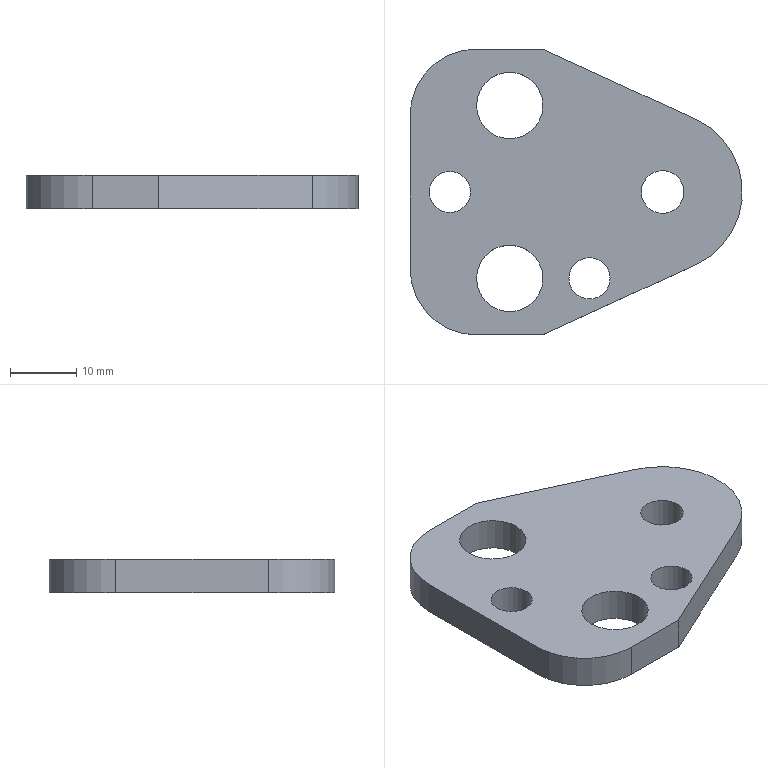Part | NX | features solid 2 | 1 solid | 15 faces | box 50 x 43 x 5 mm | volume 7113 mm3 | cylinder 8 | plane 7 | commonest cylinder face diameters 6.2 x2 10 x2 20 x2 6.4 x1 24 x1
STEP:
#1=CARTESIAN_POINT('',(-1290.413,363.428,133.));
#2=VERTEX_POINT('',#1);
#3=CARTESIAN_POINT('',(-1300.413,373.428,133.));
#4=VERTEX_POINT('',#3);
#5=CARTESIAN_POINT('',(-1290.413,373.428,133.));
#6=DIRECTION('',(0.,0.,-1.));
#7=DIRECTION('',(-1.,0.,0.));
#8=AXIS2_PLACEMENT_3D('',#5,#6,#7);
#9=CIRCLE('',#8,10.);
#10=EDGE_CURVE('',#2,#4,#9,.T.);
#11=ORIENTED_EDGE('',*,*,#10,.F.);
#12=CARTESIAN_POINT('',(-1290.413,363.428,138.));
#13=VERTEX_POINT('',#12);
#14=CARTESIAN_POINT('',(-1290.413,363.428,138.));
#15=DIRECTION('',(0.,0.,-1.));
#16=VECTOR('',#15,1000.);
#17=LINE('',#14,#16);
#18=EDGE_CURVE('',#13,#2,#17,.T.);
#19=ORIENTED_EDGE('',*,*,#18,.F.);
#20=CARTESIAN_POINT('',(-1300.413,373.428,138.));
#21=VERTEX_POINT('',#20);
#22=CARTESIAN_POINT('',(-1290.413,373.428,138.));
#23=DIRECTION('',(0.,0.,-1.));
#24=DIRECTION('',(-1.,0.,0.));
#25=AXIS2_PLACEMENT_3D('',#22,#23,#24);
#26=CIRCLE('',#25,10.);
#27=EDGE_CURVE('',#13,#21,#26,.T.);
#28=ORIENTED_EDGE('',*,*,#27,.T.);
#29=CARTESIAN_POINT('',(-1300.413,373.428,138.));
#30=DIRECTION('',(0.,0.,-1.));
#31=VECTOR('',#30,1000.);
#32=LINE('',#29,#31);
#33=EDGE_CURVE('',#21,#4,#32,.T.);
#34=ORIENTED_EDGE('',*,*,#33,.T.);
#35=EDGE_LOOP('',(#11,#19,#28,#34));
#36=FACE_BOUND('',#35,.T.);
#37=CARTESIAN_POINT('',(-1290.413,373.428,138.));
#38=DIRECTION('',(0.,0.,-1.));
#39=DIRECTION('',(-1.,0.,0.));
#40=AXIS2_PLACEMENT_3D('',#37,#38,#39);
#41=CYLINDRICAL_SURFACE('',#40,10.);
#42=ADVANCED_FACE('',(#36),#41,.T.);
#43=CARTESIAN_POINT('',(-1300.413,396.428,133.));
#44=VERTEX_POINT('',#43);
#45=CARTESIAN_POINT('',(-1300.413,396.428,133.));
#46=DIRECTION('',(0.,-1.,0.));
#47=VECTOR('',#46,1000.);
#48=LINE('',#45,#47);
#49=EDGE_CURVE('',#44,#4,#48,.T.);
#50=ORIENTED_EDGE('',*,*,#49,.T.);
#51=ORIENTED_EDGE('',*,*,#33,.F.);
#52=CARTESIAN_POINT('',(-1300.413,396.428,138.));
#53=VERTEX_POINT('',#52);
#54=CARTESIAN_POINT('',(-1300.413,396.428,138.));
#55=DIRECTION('',(0.,-1.,0.));
#56=VECTOR('',#55,1000.);
#57=LINE('',#54,#56);
#58=EDGE_CURVE('',#53,#21,#57,.T.);
#59=ORIENTED_EDGE('',*,*,#58,.F.);
#60=CARTESIAN_POINT('',(-1300.413,396.428,138.));
#61=DIRECTION('',(0.,0.,-1.));
#62=VECTOR('',#61,1000.);
#63=LINE('',#60,#62);
#64=EDGE_CURVE('',#53,#44,#63,.T.);
#65=ORIENTED_EDGE('',*,*,#64,.T.);
#66=EDGE_LOOP('',(#50,#51,#59,#65));
#67=FACE_BOUND('',#66,.T.);
#68=CARTESIAN_POINT('',(-1300.413,396.428,138.));
#69=DIRECTION('',(1.,0.,0.));
#70=DIRECTION('',(0.,1.,0.));
#71=AXIS2_PLACEMENT_3D('',#68,#69,#70);
#72=PLANE('',#71);
#73=ADVANCED_FACE('',(#67),#72,.F.);
#74=CARTESIAN_POINT('',(-1290.413,406.428,133.));
#75=VERTEX_POINT('',#74);
#76=CARTESIAN_POINT('',(-1290.413,396.428,133.));
#77=DIRECTION('',(0.,0.,-1.));
#78=DIRECTION('',(-1.,0.,0.));
#79=AXIS2_PLACEMENT_3D('',#76,#77,#78);
#80=CIRCLE('',#79,10.);
#81=EDGE_CURVE('',#44,#75,#80,.T.);
#82=ORIENTED_EDGE('',*,*,#81,.F.);
#83=ORIENTED_EDGE('',*,*,#64,.F.);
#84=CARTESIAN_POINT('',(-1290.413,406.428,138.));
#85=VERTEX_POINT('',#84);
#86=CARTESIAN_POINT('',(-1290.413,396.428,138.));
#87=DIRECTION('',(0.,0.,-1.));
#88=DIRECTION('',(-1.,0.,0.));
#89=AXIS2_PLACEMENT_3D('',#86,#87,#88);
#90=CIRCLE('',#89,10.);
#91=EDGE_CURVE('',#53,#85,#90,.T.);
#92=ORIENTED_EDGE('',*,*,#91,.T.);
#93=CARTESIAN_POINT('',(-1290.413,406.428,138.));
#94=DIRECTION('',(0.,0.,-1.));
#95=VECTOR('',#94,1000.);
#96=LINE('',#93,#95);
#97=EDGE_CURVE('',#85,#75,#96,.T.);
#98=ORIENTED_EDGE('',*,*,#97,.T.);
#99=EDGE_LOOP('',(#82,#83,#92,#98));
#100=FACE_BOUND('',#99,.T.);
#101=CARTESIAN_POINT('',(-1290.413,396.428,138.));
#102=DIRECTION('',(0.,0.,-1.));
#103=DIRECTION('',(-1.,0.,0.));
#104=AXIS2_PLACEMENT_3D('',#101,#102,#103);
#105=CYLINDRICAL_SURFACE('',#104,10.);
#106=ADVANCED_FACE('',(#100),#105,.T.);
#107=CARTESIAN_POINT('',(-1280.413,406.428,133.));
#108=VERTEX_POINT('',#107);
#109=CARTESIAN_POINT('',(-1280.413,406.428,133.));
#110=DIRECTION('',(-1.,0.,0.));
#111=VECTOR('',#110,1000.);
#112=LINE('',#109,#111);
#113=EDGE_CURVE('',#108,#75,#112,.T.);
#114=ORIENTED_EDGE('',*,*,#113,.T.);
#115=ORIENTED_EDGE('',*,*,#97,.F.);
#116=CARTESIAN_POINT('',(-1280.413,406.428,138.));
#117=VERTEX_POINT('',#116);
#118=CARTESIAN_POINT('',(-1280.413,406.428,138.));
#119=DIRECTION('',(-1.,0.,0.));
#120=VECTOR('',#119,1000.);
#121=LINE('',#118,#120);
#122=EDGE_CURVE('',#117,#85,#121,.T.);
#123=ORIENTED_EDGE('',*,*,#122,.F.);
#124=CARTESIAN_POINT('',(-1280.413,406.428,138.));
#125=DIRECTION('',(0.,0.,-1.));
#126=VECTOR('',#125,1000.);
#127=LINE('',#124,#126);
#128=EDGE_CURVE('',#117,#108,#127,.T.);
#129=ORIENTED_EDGE('',*,*,#128,.T.);
#130=EDGE_LOOP('',(#114,#115,#123,#129));
#131=FACE_BOUND('',#130,.T.);
#132=CARTESIAN_POINT('',(-1280.413,406.428,138.));
#133=DIRECTION('',(0.,-1.,0.));
#134=DIRECTION('',(1.,0.,0.));
#135=AXIS2_PLACEMENT_3D('',#132,#133,#134);
#136=PLANE('',#135);
#137=ADVANCED_FACE('',(#131),#136,.F.);
#138=CARTESIAN_POINT('',(-1257.394,395.828,133.));
#139=VERTEX_POINT('',#138);
#140=CARTESIAN_POINT('',(-1257.394,395.828,133.));
#141=DIRECTION('',(-0.9083,0.4183,0.));
#142=VECTOR('',#141,1000.);
#143=LINE('',#140,#142);
#144=EDGE_CURVE('',#139,#108,#143,.T.);
#145=ORIENTED_EDGE('',*,*,#144,.T.);
#146=ORIENTED_EDGE('',*,*,#128,.F.);
#147=CARTESIAN_POINT('',(-1257.394,395.828,138.));
#148=VERTEX_POINT('',#147);
#149=CARTESIAN_POINT('',(-1257.394,395.828,138.));
#150=DIRECTION('',(-0.9083,0.4183,0.));
#151=VECTOR('',#150,1000.);
#152=LINE('',#149,#151);
#153=EDGE_CURVE('',#148,#117,#152,.T.);
#154=ORIENTED_EDGE('',*,*,#153,.F.);
#155=CARTESIAN_POINT('',(-1257.394,395.828,138.));
#156=DIRECTION('',(0.,0.,-1.));
#157=VECTOR('',#156,1000.);
#158=LINE('',#155,#157);
#159=EDGE_CURVE('',#148,#139,#158,.T.);
#160=ORIENTED_EDGE('',*,*,#159,.T.);
#161=EDGE_LOOP('',(#145,#146,#154,#160));
#162=FACE_BOUND('',#161,.T.);
#163=CARTESIAN_POINT('',(-1257.394,395.828,138.));
#164=DIRECTION('',(-0.4183,-0.9083,0.));
#165=DIRECTION('',(0.9083,-0.4183,0.));
#166=AXIS2_PLACEMENT_3D('',#163,#164,#165);
#167=PLANE('',#166);
#168=ADVANCED_FACE('',(#162),#167,.F.);
#169=CARTESIAN_POINT('',(-1257.394,374.028,133.));
#170=VERTEX_POINT('',#169);
#171=CARTESIAN_POINT('',(-1262.413,384.928,133.));
#172=DIRECTION('',(0.,0.,-1.));
#173=DIRECTION('',(-1.,0.,0.));
#174=AXIS2_PLACEMENT_3D('',#171,#172,#173);
#175=CIRCLE('',#174,12.);
#176=EDGE_CURVE('',#139,#170,#175,.T.);
#177=ORIENTED_EDGE('',*,*,#176,.F.);
#178=ORIENTED_EDGE('',*,*,#159,.F.);
#179=CARTESIAN_POINT('',(-1257.394,374.028,138.));
#180=VERTEX_POINT('',#179);
#181=CARTESIAN_POINT('',(-1262.413,384.928,138.));
#182=DIRECTION('',(0.,0.,-1.));
#183=DIRECTION('',(-1.,0.,0.));
#184=AXIS2_PLACEMENT_3D('',#181,#182,#183);
#185=CIRCLE('',#184,12.);
#186=EDGE_CURVE('',#148,#180,#185,.T.);
#187=ORIENTED_EDGE('',*,*,#186,.T.);
#188=CARTESIAN_POINT('',(-1257.394,374.028,138.));
#189=DIRECTION('',(0.,0.,-1.));
#190=VECTOR('',#189,1000.);
#191=LINE('',#188,#190);
#192=EDGE_CURVE('',#180,#170,#191,.T.);
#193=ORIENTED_EDGE('',*,*,#192,.T.);
#194=EDGE_LOOP('',(#177,#178,#187,#193));
#195=FACE_BOUND('',#194,.T.);
#196=CARTESIAN_POINT('',(-1262.413,384.928,138.));
#197=DIRECTION('',(0.,0.,-1.));
#198=DIRECTION('',(-1.,0.,0.));
#199=AXIS2_PLACEMENT_3D('',#196,#197,#198);
#200=CYLINDRICAL_SURFACE('',#199,12.);
#201=ADVANCED_FACE('',(#195),#200,.T.);
#202=CARTESIAN_POINT('',(-1280.413,363.428,133.));
#203=VERTEX_POINT('',#202);
#204=CARTESIAN_POINT('',(-1257.394,374.028,133.));
#205=DIRECTION('',(-0.9083,-0.4183,0.));
#206=VECTOR('',#205,1000.);
#207=LINE('',#204,#206);
#208=EDGE_CURVE('',#170,#203,#207,.T.);
#209=ORIENTED_EDGE('',*,*,#208,.F.);
#210=ORIENTED_EDGE('',*,*,#192,.F.);
#211=CARTESIAN_POINT('',(-1280.413,363.428,138.));
#212=VERTEX_POINT('',#211);
#213=CARTESIAN_POINT('',(-1257.394,374.028,138.));
#214=DIRECTION('',(-0.9083,-0.4183,0.));
#215=VECTOR('',#214,1000.);
#216=LINE('',#213,#215);
#217=EDGE_CURVE('',#180,#212,#216,.T.);
#218=ORIENTED_EDGE('',*,*,#217,.T.);
#219=CARTESIAN_POINT('',(-1280.413,363.428,138.));
#220=DIRECTION('',(0.,0.,-1.));
#221=VECTOR('',#220,1000.);
#222=LINE('',#219,#221);
#223=EDGE_CURVE('',#212,#203,#222,.T.);
#224=ORIENTED_EDGE('',*,*,#223,.T.);
#225=EDGE_LOOP('',(#209,#210,#218,#224));
#226=FACE_BOUND('',#225,.T.);
#227=CARTESIAN_POINT('',(-1257.394,374.028,138.));
#228=DIRECTION('',(0.4183,-0.9083,0.));
#229=DIRECTION('',(0.9083,0.4183,0.));
#230=AXIS2_PLACEMENT_3D('',#227,#228,#229);
#231=PLANE('',#230);
#232=ADVANCED_FACE('',(#226),#231,.T.);
#233=CARTESIAN_POINT('',(-1280.413,363.428,133.));
#234=DIRECTION('',(-1.,0.,0.));
#235=VECTOR('',#234,1000.);
#236=LINE('',#233,#235);
#237=EDGE_CURVE('',#203,#2,#236,.T.);
#238=ORIENTED_EDGE('',*,*,#237,.F.);
#239=ORIENTED_EDGE('',*,*,#223,.F.);
#240=CARTESIAN_POINT('',(-1280.413,363.428,138.));
#241=DIRECTION('',(-1.,0.,0.));
#242=VECTOR('',#241,1000.);
#243=LINE('',#240,#242);
#244=EDGE_CURVE('',#212,#13,#243,.T.);
#245=ORIENTED_EDGE('',*,*,#244,.T.);
#246=ORIENTED_EDGE('',*,*,#18,.T.);
#247=EDGE_LOOP('',(#238,#239,#245,#246));
#248=FACE_BOUND('',#247,.T.);
#249=CARTESIAN_POINT('',(-1280.413,363.428,138.));
#250=DIRECTION('',(0.,-1.,0.));
#251=DIRECTION('',(1.,0.,0.));
#252=AXIS2_PLACEMENT_3D('',#249,#250,#251);
#253=PLANE('',#252);
#254=ADVANCED_FACE('',(#248),#253,.T.);
#255=CARTESIAN_POINT('',(-1290.413,397.928,138.));
#256=VERTEX_POINT('',#255);
#257=CARTESIAN_POINT('',(-1285.413,397.928,138.));
#258=DIRECTION('',(0.,0.,-1.));
#259=DIRECTION('',(-1.,0.,0.));
#260=AXIS2_PLACEMENT_3D('',#257,#258,#259);
#261=CIRCLE('',#260,5.);
#262=EDGE_CURVE('',#256,#256,#261,.T.);
#263=ORIENTED_EDGE('',*,*,#262,.T.);
#264=EDGE_LOOP('',(#263));
#265=FACE_BOUND('',#264,.T.);
#266=CARTESIAN_POINT('',(-1290.413,371.928,138.));
#267=VERTEX_POINT('',#266);
#268=CARTESIAN_POINT('',(-1285.413,371.928,138.));
#269=DIRECTION('',(0.,0.,-1.));
#270=DIRECTION('',(-1.,0.,0.));
#271=AXIS2_PLACEMENT_3D('',#268,#269,#270);
#272=CIRCLE('',#271,5.);
#273=EDGE_CURVE('',#267,#267,#272,.T.);
#274=ORIENTED_EDGE('',*,*,#273,.T.);
#275=EDGE_LOOP('',(#274));
#276=FACE_BOUND('',#275,.T.);
#277=CARTESIAN_POINT('',(-1265.613,384.928,138.));
#278=VERTEX_POINT('',#277);
#279=CARTESIAN_POINT('',(-1262.413,384.928,138.));
#280=DIRECTION('',(0.,0.,-1.));
#281=DIRECTION('',(-1.,0.,0.));
#282=AXIS2_PLACEMENT_3D('',#279,#280,#281);
#283=CIRCLE('',#282,3.2);
#284=EDGE_CURVE('',#278,#278,#283,.T.);
#285=ORIENTED_EDGE('',*,*,#284,.T.);
#286=EDGE_LOOP('',(#285));
#287=FACE_BOUND('',#286,.T.);
#288=CARTESIAN_POINT('',(-1276.513,371.928,138.));
#289=VERTEX_POINT('',#288);
#290=CARTESIAN_POINT('',(-1273.413,371.928,138.));
#291=DIRECTION('',(0.,0.,-1.));
#292=DIRECTION('',(-1.,0.,0.));
#293=AXIS2_PLACEMENT_3D('',#290,#291,#292);
#294=CIRCLE('',#293,3.1);
#295=EDGE_CURVE('',#289,#289,#294,.T.);
#296=ORIENTED_EDGE('',*,*,#295,.T.);
#297=EDGE_LOOP('',(#296));
#298=FACE_BOUND('',#297,.T.);
#299=CARTESIAN_POINT('',(-1297.513,384.928,138.));
#300=VERTEX_POINT('',#299);
#301=CARTESIAN_POINT('',(-1294.413,384.928,138.));
#302=DIRECTION('',(0.,0.,-1.));
#303=DIRECTION('',(-1.,0.,0.));
#304=AXIS2_PLACEMENT_3D('',#301,#302,#303);
#305=CIRCLE('',#304,3.1);
#306=EDGE_CURVE('',#300,#300,#305,.T.);
#307=ORIENTED_EDGE('',*,*,#306,.T.);
#308=EDGE_LOOP('',(#307));
#309=FACE_BOUND('',#308,.T.);
#310=ORIENTED_EDGE('',*,*,#27,.F.);
#311=ORIENTED_EDGE('',*,*,#244,.F.);
#312=ORIENTED_EDGE('',*,*,#217,.F.);
#313=ORIENTED_EDGE('',*,*,#186,.F.);
#314=ORIENTED_EDGE('',*,*,#153,.T.);
#315=ORIENTED_EDGE('',*,*,#122,.T.);
#316=ORIENTED_EDGE('',*,*,#91,.F.);
#317=ORIENTED_EDGE('',*,*,#58,.T.);
#318=EDGE_LOOP('',(#310,#311,#312,#313,#314,#315,#316,#317));
#319=FACE_BOUND('',#318,.T.);
#320=CARTESIAN_POINT('',(-1290.413,373.428,138.));
#321=DIRECTION('',(0.,0.,-1.));
#322=DIRECTION('',(-1.,0.,0.));
#323=AXIS2_PLACEMENT_3D('',#320,#321,#322);
#324=PLANE('',#323);
#325=ADVANCED_FACE('',(#265,#276,#287,#298,#309,#319),#324,.F.);
#326=CARTESIAN_POINT('',(-1290.413,397.928,133.));
#327=VERTEX_POINT('',#326);
#328=CARTESIAN_POINT('',(-1285.413,397.928,133.));
#329=DIRECTION('',(0.,0.,-1.));
#330=DIRECTION('',(-1.,0.,0.));
#331=AXIS2_PLACEMENT_3D('',#328,#329,#330);
#332=CIRCLE('',#331,5.);
#333=EDGE_CURVE('',#327,#327,#332,.T.);
#334=ORIENTED_EDGE('',*,*,#333,.F.);
#335=EDGE_LOOP('',(#334));
#336=FACE_BOUND('',#335,.T.);
#337=CARTESIAN_POINT('',(-1290.413,371.928,133.));
#338=VERTEX_POINT('',#337);
#339=CARTESIAN_POINT('',(-1285.413,371.928,133.));
#340=DIRECTION('',(0.,0.,-1.));
#341=DIRECTION('',(-1.,0.,0.));
#342=AXIS2_PLACEMENT_3D('',#339,#340,#341);
#343=CIRCLE('',#342,5.);
#344=EDGE_CURVE('',#338,#338,#343,.T.);
#345=ORIENTED_EDGE('',*,*,#344,.F.);
#346=EDGE_LOOP('',(#345));
#347=FACE_BOUND('',#346,.T.);
#348=CARTESIAN_POINT('',(-1265.613,384.928,133.));
#349=VERTEX_POINT('',#348);
#350=CARTESIAN_POINT('',(-1262.413,384.928,133.));
#351=DIRECTION('',(0.,0.,-1.));
#352=DIRECTION('',(-1.,0.,0.));
#353=AXIS2_PLACEMENT_3D('',#350,#351,#352);
#354=CIRCLE('',#353,3.2);
#355=EDGE_CURVE('',#349,#349,#354,.T.);
#356=ORIENTED_EDGE('',*,*,#355,.F.);
#357=EDGE_LOOP('',(#356));
#358=FACE_BOUND('',#357,.T.);
#359=CARTESIAN_POINT('',(-1276.513,371.928,133.));
#360=VERTEX_POINT('',#359);
#361=CARTESIAN_POINT('',(-1273.413,371.928,133.));
#362=DIRECTION('',(0.,0.,-1.));
#363=DIRECTION('',(-1.,0.,0.));
#364=AXIS2_PLACEMENT_3D('',#361,#362,#363);
#365=CIRCLE('',#364,3.1);
#366=EDGE_CURVE('',#360,#360,#365,.T.);
#367=ORIENTED_EDGE('',*,*,#366,.F.);
#368=EDGE_LOOP('',(#367));
#369=FACE_BOUND('',#368,.T.);
#370=CARTESIAN_POINT('',(-1297.513,384.928,133.));
#371=VERTEX_POINT('',#370);
#372=CARTESIAN_POINT('',(-1294.413,384.928,133.));
#373=DIRECTION('',(0.,0.,-1.));
#374=DIRECTION('',(-1.,0.,0.));
#375=AXIS2_PLACEMENT_3D('',#372,#373,#374);
#376=CIRCLE('',#375,3.1);
#377=EDGE_CURVE('',#371,#371,#376,.T.);
#378=ORIENTED_EDGE('',*,*,#377,.F.);
#379=EDGE_LOOP('',(#378));
#380=FACE_BOUND('',#379,.T.);
#381=ORIENTED_EDGE('',*,*,#10,.T.);
#382=ORIENTED_EDGE('',*,*,#49,.F.);
#383=ORIENTED_EDGE('',*,*,#81,.T.);
#384=ORIENTED_EDGE('',*,*,#113,.F.);
#385=ORIENTED_EDGE('',*,*,#144,.F.);
#386=ORIENTED_EDGE('',*,*,#176,.T.);
#387=ORIENTED_EDGE('',*,*,#208,.T.);
#388=ORIENTED_EDGE('',*,*,#237,.T.);
#389=EDGE_LOOP('',(#381,#382,#383,#384,#385,#386,#387,#388));
#390=FACE_BOUND('',#389,.T.);
#391=CARTESIAN_POINT('',(-1290.413,373.428,133.));
#392=DIRECTION('',(0.,0.,-1.));
#393=DIRECTION('',(-1.,0.,0.));
#394=AXIS2_PLACEMENT_3D('',#391,#392,#393);
#395=PLANE('',#394);
#396=ADVANCED_FACE('',(#336,#347,#358,#369,#380,#390),#395,.T.);
#397=ORIENTED_EDGE('',*,*,#377,.T.);
#398=EDGE_LOOP('',(#397));
#399=FACE_BOUND('',#398,.T.);
#400=ORIENTED_EDGE('',*,*,#306,.F.);
#401=EDGE_LOOP('',(#400));
#402=FACE_BOUND('',#401,.T.);
#403=CARTESIAN_POINT('',(-1294.413,384.928,138.));
#404=DIRECTION('',(0.,0.,-1.));
#405=DIRECTION('',(-1.,0.,0.));
#406=AXIS2_PLACEMENT_3D('',#403,#404,#405);
#407=CYLINDRICAL_SURFACE('',#406,3.1);
#408=ADVANCED_FACE('',(#399,#402),#407,.F.);
#409=ORIENTED_EDGE('',*,*,#366,.T.);
#410=EDGE_LOOP('',(#409));
#411=FACE_BOUND('',#410,.T.);
#412=ORIENTED_EDGE('',*,*,#295,.F.);
#413=EDGE_LOOP('',(#412));
#414=FACE_BOUND('',#413,.T.);
#415=CARTESIAN_POINT('',(-1273.413,371.928,138.));
#416=DIRECTION('',(0.,0.,-1.));
#417=DIRECTION('',(-1.,0.,0.));
#418=AXIS2_PLACEMENT_3D('',#415,#416,#417);
#419=CYLINDRICAL_SURFACE('',#418,3.1);
#420=ADVANCED_FACE('',(#411,#414),#419,.F.);
#421=ORIENTED_EDGE('',*,*,#355,.T.);
#422=EDGE_LOOP('',(#421));
#423=FACE_BOUND('',#422,.T.);
#424=ORIENTED_EDGE('',*,*,#284,.F.);
#425=EDGE_LOOP('',(#424));
#426=FACE_BOUND('',#425,.T.);
#427=CARTESIAN_POINT('',(-1262.413,384.928,138.));
#428=DIRECTION('',(0.,0.,-1.));
#429=DIRECTION('',(-1.,0.,0.));
#430=AXIS2_PLACEMENT_3D('',#427,#428,#429);
#431=CYLINDRICAL_SURFACE('',#430,3.2);
#432=ADVANCED_FACE('',(#423,#426),#431,.F.);
#433=ORIENTED_EDGE('',*,*,#344,.T.);
#434=EDGE_LOOP('',(#433));
#435=FACE_BOUND('',#434,.T.);
#436=ORIENTED_EDGE('',*,*,#273,.F.);
#437=EDGE_LOOP('',(#436));
#438=FACE_BOUND('',#437,.T.);
#439=CARTESIAN_POINT('',(-1285.413,371.928,138.));
#440=DIRECTION('',(0.,0.,-1.));
#441=DIRECTION('',(-1.,0.,0.));
#442=AXIS2_PLACEMENT_3D('',#439,#440,#441);
#443=CYLINDRICAL_SURFACE('',#442,5.);
#444=ADVANCED_FACE('',(#435,#438),#443,.F.);
#445=ORIENTED_EDGE('',*,*,#333,.T.);
#446=EDGE_LOOP('',(#445));
#447=FACE_BOUND('',#446,.T.);
#448=ORIENTED_EDGE('',*,*,#262,.F.);
#449=EDGE_LOOP('',(#448));
#450=FACE_BOUND('',#449,.T.);
#451=CARTESIAN_POINT('',(-1285.413,397.928,138.));
#452=DIRECTION('',(0.,0.,-1.));
#453=DIRECTION('',(-1.,0.,0.));
#454=AXIS2_PLACEMENT_3D('',#451,#452,#453);
#455=CYLINDRICAL_SURFACE('',#454,5.);
#456=ADVANCED_FACE('',(#447,#450),#455,.F.);
#457=CLOSED_SHELL('',(#42,#73,#106,#137,#168,#201,#232,#254,#325,#396,#408,#420,#432,#444,#456));
#458=MANIFOLD_SOLID_BREP('',#457);
#459=(LENGTH_UNIT()NAMED_UNIT(*)SI_UNIT(.MILLI.,.METRE.));
#460=UNCERTAINTY_MEASURE_WITH_UNIT(LENGTH_MEASURE(0.00001),#459,'','');
#461=(NAMED_UNIT(*)PLANE_ANGLE_UNIT()SI_UNIT($,.RADIAN.));
#462=(NAMED_UNIT(*)SI_UNIT($,.STERADIAN.)SOLID_ANGLE_UNIT());
#463=(GEOMETRIC_REPRESENTATION_CONTEXT(3)GLOBAL_UNCERTAINTY_ASSIGNED_CONTEXT((#460))GLOBAL_UNIT_ASSIGNED_CONTEXT((#459,#461,#462))REPRESENTATION_CONTEXT('',''));
#464=ADVANCED_BREP_SHAPE_REPRESENTATION('',(#458),#463);